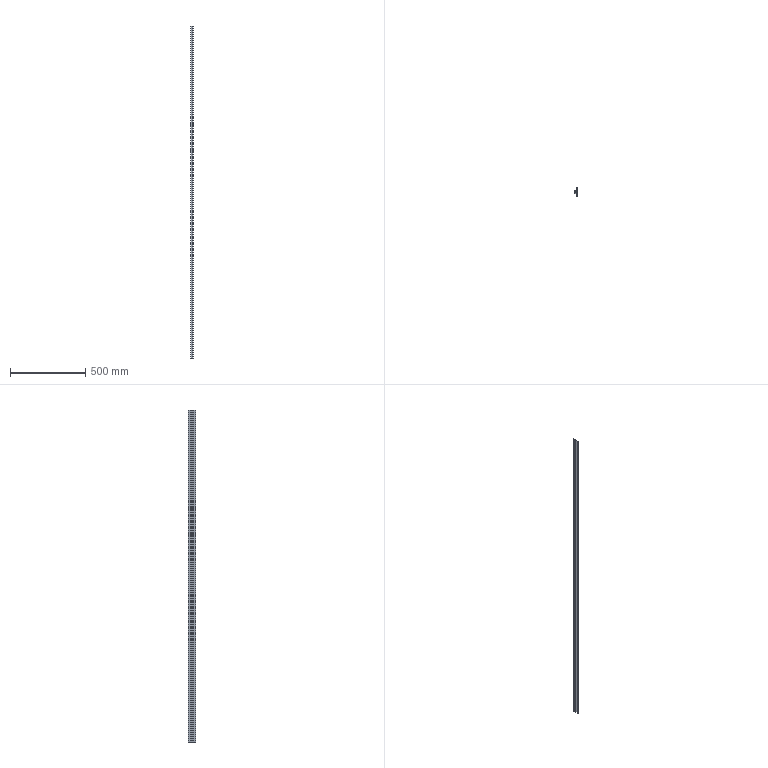Part | STEP file | Guide wheel mechanism revised.sldasm-Part-78 | 1 solid | 22 faces | box 14 x 50 x 2200 mm | volume 559680 mm3 | plane 22
STEP:
#1=CARTESIAN_POINT('',(0.,-7.,-1100.));
#2=VERTEX_POINT('',#1);
#3=CARTESIAN_POINT('',(-8.,-7.,-1100.));
#4=VERTEX_POINT('',#3);
#5=CARTESIAN_POINT('',(-8.,-7.,-1100.));
#6=DIRECTION('',(-1.,0.,0.));
#7=VECTOR('',#6,1000.);
#8=LINE('',#5,#7);
#9=EDGE_CURVE('',#2,#4,#8,.T.);
#10=ORIENTED_EDGE('',*,*,#9,.T.);
#11=CARTESIAN_POINT('',(-8.,-7.,1100.));
#12=VERTEX_POINT('',#11);
#13=CARTESIAN_POINT('',(-8.,-7.,1100.));
#14=DIRECTION('',(0.,0.,-1.));
#15=VECTOR('',#14,1000.);
#16=LINE('',#13,#15);
#17=EDGE_CURVE('',#12,#4,#16,.T.);
#18=ORIENTED_EDGE('',*,*,#17,.F.);
#19=CARTESIAN_POINT('',(0.,-7.,1100.));
#20=VERTEX_POINT('',#19);
#21=CARTESIAN_POINT('',(-8.,-7.,1100.));
#22=DIRECTION('',(-1.,0.,0.));
#23=VECTOR('',#22,1000.);
#24=LINE('',#21,#23);
#25=EDGE_CURVE('',#20,#12,#24,.T.);
#26=ORIENTED_EDGE('',*,*,#25,.F.);
#27=CARTESIAN_POINT('',(0.,-7.,1100.));
#28=DIRECTION('',(0.,0.,-1.));
#29=VECTOR('',#28,1000.);
#30=LINE('',#27,#29);
#31=EDGE_CURVE('',#20,#2,#30,.T.);
#32=ORIENTED_EDGE('',*,*,#31,.T.);
#33=EDGE_LOOP('',(#10,#18,#26,#32));
#34=FACE_OUTER_BOUND('',#33,.T.);
#35=CARTESIAN_POINT('',(-8.,-7.,1100.));
#36=DIRECTION('',(0.,-1.,0.));
#37=DIRECTION('',(1.,0.,0.));
#38=AXIS2_PLACEMENT_3D('',#35,#36,#37);
#39=PLANE('',#38);
#40=ADVANCED_FACE('',(#34),#39,.F.);
#41=CARTESIAN_POINT('',(-8.,-4.6,-1100.));
#42=VERTEX_POINT('',#41);
#43=CARTESIAN_POINT('',(-8.,-4.6,-1100.));
#44=DIRECTION('',(0.,1.,0.));
#45=VECTOR('',#44,1000.);
#46=LINE('',#43,#45);
#47=EDGE_CURVE('',#4,#42,#46,.T.);
#48=ORIENTED_EDGE('',*,*,#47,.T.);
#49=CARTESIAN_POINT('',(-8.,-4.6,1100.));
#50=VERTEX_POINT('',#49);
#51=CARTESIAN_POINT('',(-8.,-4.6,1100.));
#52=DIRECTION('',(0.,0.,-1.));
#53=VECTOR('',#52,1000.);
#54=LINE('',#51,#53);
#55=EDGE_CURVE('',#50,#42,#54,.T.);
#56=ORIENTED_EDGE('',*,*,#55,.F.);
#57=CARTESIAN_POINT('',(-8.,-4.6,1100.));
#58=DIRECTION('',(0.,1.,0.));
#59=VECTOR('',#58,1000.);
#60=LINE('',#57,#59);
#61=EDGE_CURVE('',#12,#50,#60,.T.);
#62=ORIENTED_EDGE('',*,*,#61,.F.);
#63=ORIENTED_EDGE('',*,*,#17,.T.);
#64=EDGE_LOOP('',(#48,#56,#62,#63));
#65=FACE_OUTER_BOUND('',#64,.T.);
#66=CARTESIAN_POINT('',(-8.,-4.6,1100.));
#67=DIRECTION('',(-1.,0.,0.));
#68=DIRECTION('',(0.,0.,1.));
#69=AXIS2_PLACEMENT_3D('',#66,#67,#68);
#70=PLANE('',#69);
#71=ADVANCED_FACE('',(#65),#70,.F.);
#72=CARTESIAN_POINT('',(-11.,-4.6,-1100.));
#73=VERTEX_POINT('',#72);
#74=CARTESIAN_POINT('',(-11.,-4.6,-1100.));
#75=DIRECTION('',(-1.,0.,0.));
#76=VECTOR('',#75,1000.);
#77=LINE('',#74,#76);
#78=EDGE_CURVE('',#42,#73,#77,.T.);
#79=ORIENTED_EDGE('',*,*,#78,.T.);
#80=CARTESIAN_POINT('',(-11.,-4.6,1100.));
#81=VERTEX_POINT('',#80);
#82=CARTESIAN_POINT('',(-11.,-4.6,1100.));
#83=DIRECTION('',(0.,0.,-1.));
#84=VECTOR('',#83,1000.);
#85=LINE('',#82,#84);
#86=EDGE_CURVE('',#81,#73,#85,.T.);
#87=ORIENTED_EDGE('',*,*,#86,.F.);
#88=CARTESIAN_POINT('',(-11.,-4.6,1100.));
#89=DIRECTION('',(-1.,0.,0.));
#90=VECTOR('',#89,1000.);
#91=LINE('',#88,#90);
#92=EDGE_CURVE('',#50,#81,#91,.T.);
#93=ORIENTED_EDGE('',*,*,#92,.F.);
#94=ORIENTED_EDGE('',*,*,#55,.T.);
#95=EDGE_LOOP('',(#79,#87,#93,#94));
#96=FACE_OUTER_BOUND('',#95,.T.);
#97=CARTESIAN_POINT('',(-11.,-4.6,1100.));
#98=DIRECTION('',(0.,-1.,0.));
#99=DIRECTION('',(0.,0.,-1.));
#100=AXIS2_PLACEMENT_3D('',#97,#98,#99);
#101=PLANE('',#100);
#102=ADVANCED_FACE('',(#96),#101,.F.);
#103=CARTESIAN_POINT('',(-11.,-10.,-1100.));
#104=VERTEX_POINT('',#103);
#105=CARTESIAN_POINT('',(-11.,-10.,-1100.));
#106=DIRECTION('',(0.,-1.,0.));
#107=VECTOR('',#106,1000.);
#108=LINE('',#105,#107);
#109=EDGE_CURVE('',#73,#104,#108,.T.);
#110=ORIENTED_EDGE('',*,*,#109,.T.);
#111=CARTESIAN_POINT('',(-11.,-10.,1100.));
#112=VERTEX_POINT('',#111);
#113=CARTESIAN_POINT('',(-11.,-10.,1100.));
#114=DIRECTION('',(0.,0.,-1.));
#115=VECTOR('',#114,1000.);
#116=LINE('',#113,#115);
#117=EDGE_CURVE('',#112,#104,#116,.T.);
#118=ORIENTED_EDGE('',*,*,#117,.F.);
#119=CARTESIAN_POINT('',(-11.,-10.,1100.));
#120=DIRECTION('',(0.,-1.,0.));
#121=VECTOR('',#120,1000.);
#122=LINE('',#119,#121);
#123=EDGE_CURVE('',#81,#112,#122,.T.);
#124=ORIENTED_EDGE('',*,*,#123,.F.);
#125=ORIENTED_EDGE('',*,*,#86,.T.);
#126=EDGE_LOOP('',(#110,#118,#124,#125));
#127=FACE_OUTER_BOUND('',#126,.T.);
#128=CARTESIAN_POINT('',(-11.,-10.,1100.));
#129=DIRECTION('',(1.,0.,0.));
#130=DIRECTION('',(0.,1.,0.));
#131=AXIS2_PLACEMENT_3D('',#128,#129,#130);
#132=PLANE('',#131);
#133=ADVANCED_FACE('',(#127),#132,.F.);
#134=CARTESIAN_POINT('',(0.,-10.,-1100.));
#135=VERTEX_POINT('',#134);
#136=CARTESIAN_POINT('',(0.,-10.,-1100.));
#137=DIRECTION('',(1.,0.,0.));
#138=VECTOR('',#137,1000.);
#139=LINE('',#136,#138);
#140=EDGE_CURVE('',#104,#135,#139,.T.);
#141=ORIENTED_EDGE('',*,*,#140,.T.);
#142=CARTESIAN_POINT('',(0.,-10.,1100.));
#143=VERTEX_POINT('',#142);
#144=CARTESIAN_POINT('',(0.,-10.,1100.));
#145=DIRECTION('',(0.,0.,-1.));
#146=VECTOR('',#145,1000.);
#147=LINE('',#144,#146);
#148=EDGE_CURVE('',#143,#135,#147,.T.);
#149=ORIENTED_EDGE('',*,*,#148,.F.);
#150=CARTESIAN_POINT('',(0.,-10.,1100.));
#151=DIRECTION('',(1.,0.,0.));
#152=VECTOR('',#151,1000.);
#153=LINE('',#150,#152);
#154=EDGE_CURVE('',#112,#143,#153,.T.);
#155=ORIENTED_EDGE('',*,*,#154,.F.);
#156=ORIENTED_EDGE('',*,*,#117,.T.);
#157=EDGE_LOOP('',(#141,#149,#155,#156));
#158=FACE_OUTER_BOUND('',#157,.T.);
#159=CARTESIAN_POINT('',(0.,-10.,1100.));
#160=DIRECTION('',(0.,1.,0.));
#161=DIRECTION('',(-1.,0.,0.));
#162=AXIS2_PLACEMENT_3D('',#159,#160,#161);
#163=PLANE('',#162);
#164=ADVANCED_FACE('',(#158),#163,.F.);
#165=CARTESIAN_POINT('',(0.,-21.,-1100.));
#166=VERTEX_POINT('',#165);
#167=CARTESIAN_POINT('',(0.,-21.,-1100.));
#168=DIRECTION('',(0.,-1.,0.));
#169=VECTOR('',#168,1000.);
#170=LINE('',#167,#169);
#171=EDGE_CURVE('',#135,#166,#170,.T.);
#172=ORIENTED_EDGE('',*,*,#171,.T.);
#173=CARTESIAN_POINT('',(0.,-21.,1100.));
#174=VERTEX_POINT('',#173);
#175=CARTESIAN_POINT('',(0.,-21.,1100.));
#176=DIRECTION('',(0.,0.,-1.));
#177=VECTOR('',#176,1000.);
#178=LINE('',#175,#177);
#179=EDGE_CURVE('',#174,#166,#178,.T.);
#180=ORIENTED_EDGE('',*,*,#179,.F.);
#181=CARTESIAN_POINT('',(0.,-21.,1100.));
#182=DIRECTION('',(0.,-1.,0.));
#183=VECTOR('',#182,1000.);
#184=LINE('',#181,#183);
#185=EDGE_CURVE('',#143,#174,#184,.T.);
#186=ORIENTED_EDGE('',*,*,#185,.F.);
#187=ORIENTED_EDGE('',*,*,#148,.T.);
#188=EDGE_LOOP('',(#172,#180,#186,#187));
#189=FACE_OUTER_BOUND('',#188,.T.);
#190=CARTESIAN_POINT('',(0.,-21.,1100.));
#191=DIRECTION('',(1.,0.,0.));
#192=DIRECTION('',(0.,1.,0.));
#193=AXIS2_PLACEMENT_3D('',#190,#191,#192);
#194=PLANE('',#193);
#195=ADVANCED_FACE('',(#189),#194,.F.);
#196=CARTESIAN_POINT('',(-3.,-21.,-1100.));
#197=VERTEX_POINT('',#196);
#198=CARTESIAN_POINT('',(-3.,-21.,-1100.));
#199=DIRECTION('',(-1.,0.,0.));
#200=VECTOR('',#199,1000.);
#201=LINE('',#198,#200);
#202=EDGE_CURVE('',#166,#197,#201,.T.);
#203=ORIENTED_EDGE('',*,*,#202,.T.);
#204=CARTESIAN_POINT('',(-3.,-21.,1100.));
#205=VERTEX_POINT('',#204);
#206=CARTESIAN_POINT('',(-3.,-21.,1100.));
#207=DIRECTION('',(0.,0.,-1.));
#208=VECTOR('',#207,1000.);
#209=LINE('',#206,#208);
#210=EDGE_CURVE('',#205,#197,#209,.T.);
#211=ORIENTED_EDGE('',*,*,#210,.F.);
#212=CARTESIAN_POINT('',(-3.,-21.,1100.));
#213=DIRECTION('',(-1.,0.,0.));
#214=VECTOR('',#213,1000.);
#215=LINE('',#212,#214);
#216=EDGE_CURVE('',#174,#205,#215,.T.);
#217=ORIENTED_EDGE('',*,*,#216,.F.);
#218=ORIENTED_EDGE('',*,*,#179,.T.);
#219=EDGE_LOOP('',(#203,#211,#217,#218));
#220=FACE_OUTER_BOUND('',#219,.T.);
#221=CARTESIAN_POINT('',(-3.,-21.,1100.));
#222=DIRECTION('',(0.,-1.,0.));
#223=DIRECTION('',(1.,0.,0.));
#224=AXIS2_PLACEMENT_3D('',#221,#222,#223);
#225=PLANE('',#224);
#226=ADVANCED_FACE('',(#220),#225,.F.);
#227=CARTESIAN_POINT('',(-3.,-25.,-1100.));
#228=VERTEX_POINT('',#227);
#229=CARTESIAN_POINT('',(-3.,-25.,-1100.));
#230=DIRECTION('',(0.,-1.,0.));
#231=VECTOR('',#230,1000.);
#232=LINE('',#229,#231);
#233=EDGE_CURVE('',#197,#228,#232,.T.);
#234=ORIENTED_EDGE('',*,*,#233,.T.);
#235=CARTESIAN_POINT('',(-3.,-25.,1100.));
#236=VERTEX_POINT('',#235);
#237=CARTESIAN_POINT('',(-3.,-25.,1100.));
#238=DIRECTION('',(0.,0.,-1.));
#239=VECTOR('',#238,1000.);
#240=LINE('',#237,#239);
#241=EDGE_CURVE('',#236,#228,#240,.T.);
#242=ORIENTED_EDGE('',*,*,#241,.F.);
#243=CARTESIAN_POINT('',(-3.,-25.,1100.));
#244=DIRECTION('',(0.,-1.,0.));
#245=VECTOR('',#244,1000.);
#246=LINE('',#243,#245);
#247=EDGE_CURVE('',#205,#236,#246,.T.);
#248=ORIENTED_EDGE('',*,*,#247,.F.);
#249=ORIENTED_EDGE('',*,*,#210,.T.);
#250=EDGE_LOOP('',(#234,#242,#248,#249));
#251=FACE_OUTER_BOUND('',#250,.T.);
#252=CARTESIAN_POINT('',(-3.,-25.,1100.));
#253=DIRECTION('',(1.,0.,0.));
#254=DIRECTION('',(0.,0.,-1.));
#255=AXIS2_PLACEMENT_3D('',#252,#253,#254);
#256=PLANE('',#255);
#257=ADVANCED_FACE('',(#251),#256,.F.);
#258=CARTESIAN_POINT('',(3.,-25.,-1100.));
#259=VERTEX_POINT('',#258);
#260=CARTESIAN_POINT('',(3.,-25.,-1100.));
#261=DIRECTION('',(1.,0.,0.));
#262=VECTOR('',#261,1000.);
#263=LINE('',#260,#262);
#264=EDGE_CURVE('',#228,#259,#263,.T.);
#265=ORIENTED_EDGE('',*,*,#264,.T.);
#266=CARTESIAN_POINT('',(3.,-25.,1100.));
#267=VERTEX_POINT('',#266);
#268=CARTESIAN_POINT('',(3.,-25.,1100.));
#269=DIRECTION('',(0.,0.,-1.));
#270=VECTOR('',#269,1000.);
#271=LINE('',#268,#270);
#272=EDGE_CURVE('',#267,#259,#271,.T.);
#273=ORIENTED_EDGE('',*,*,#272,.F.);
#274=CARTESIAN_POINT('',(3.,-25.,1100.));
#275=DIRECTION('',(1.,0.,0.));
#276=VECTOR('',#275,1000.);
#277=LINE('',#274,#276);
#278=EDGE_CURVE('',#236,#267,#277,.T.);
#279=ORIENTED_EDGE('',*,*,#278,.F.);
#280=ORIENTED_EDGE('',*,*,#241,.T.);
#281=EDGE_LOOP('',(#265,#273,#279,#280));
#282=FACE_OUTER_BOUND('',#281,.T.);
#283=CARTESIAN_POINT('',(3.,-25.,1100.));
#284=DIRECTION('',(0.,1.,0.));
#285=DIRECTION('',(0.,0.,1.));
#286=AXIS2_PLACEMENT_3D('',#283,#284,#285);
#287=PLANE('',#286);
#288=ADVANCED_FACE('',(#282),#287,.F.);
#289=CARTESIAN_POINT('',(3.,25.,-1100.));
#290=VERTEX_POINT('',#289);
#291=CARTESIAN_POINT('',(3.,-25.,-1100.));
#292=DIRECTION('',(0.,1.,0.));
#293=VECTOR('',#292,1000.);
#294=LINE('',#291,#293);
#295=EDGE_CURVE('',#259,#290,#294,.T.);
#296=ORIENTED_EDGE('',*,*,#295,.T.);
#297=CARTESIAN_POINT('',(3.,25.,1100.));
#298=VERTEX_POINT('',#297);
#299=CARTESIAN_POINT('',(3.,25.,1100.));
#300=DIRECTION('',(0.,0.,-1.));
#301=VECTOR('',#300,1000.);
#302=LINE('',#299,#301);
#303=EDGE_CURVE('',#298,#290,#302,.T.);
#304=ORIENTED_EDGE('',*,*,#303,.F.);
#305=CARTESIAN_POINT('',(3.,-25.,1100.));
#306=DIRECTION('',(0.,1.,0.));
#307=VECTOR('',#306,1000.);
#308=LINE('',#305,#307);
#309=EDGE_CURVE('',#267,#298,#308,.T.);
#310=ORIENTED_EDGE('',*,*,#309,.F.);
#311=ORIENTED_EDGE('',*,*,#272,.T.);
#312=EDGE_LOOP('',(#296,#304,#310,#311));
#313=FACE_OUTER_BOUND('',#312,.T.);
#314=CARTESIAN_POINT('',(3.,-25.,1100.));
#315=DIRECTION('',(-1.,0.,0.));
#316=DIRECTION('',(0.,0.,1.));
#317=AXIS2_PLACEMENT_3D('',#314,#315,#316);
#318=PLANE('',#317);
#319=ADVANCED_FACE('',(#313),#318,.F.);
#320=CARTESIAN_POINT('',(-3.,25.,-1100.));
#321=VERTEX_POINT('',#320);
#322=CARTESIAN_POINT('',(3.,25.,-1100.));
#323=DIRECTION('',(-1.,0.,0.));
#324=VECTOR('',#323,1000.);
#325=LINE('',#322,#324);
#326=EDGE_CURVE('',#290,#321,#325,.T.);
#327=ORIENTED_EDGE('',*,*,#326,.T.);
#328=CARTESIAN_POINT('',(-3.,25.,1100.));
#329=VERTEX_POINT('',#328);
#330=CARTESIAN_POINT('',(-3.,25.,1100.));
#331=DIRECTION('',(0.,0.,-1.));
#332=VECTOR('',#331,1000.);
#333=LINE('',#330,#332);
#334=EDGE_CURVE('',#329,#321,#333,.T.);
#335=ORIENTED_EDGE('',*,*,#334,.F.);
#336=CARTESIAN_POINT('',(3.,25.,1100.));
#337=DIRECTION('',(-1.,0.,0.));
#338=VECTOR('',#337,1000.);
#339=LINE('',#336,#338);
#340=EDGE_CURVE('',#298,#329,#339,.T.);
#341=ORIENTED_EDGE('',*,*,#340,.F.);
#342=ORIENTED_EDGE('',*,*,#303,.T.);
#343=EDGE_LOOP('',(#327,#335,#341,#342));
#344=FACE_OUTER_BOUND('',#343,.T.);
#345=CARTESIAN_POINT('',(3.,25.,1100.));
#346=DIRECTION('',(0.,-1.,0.));
#347=DIRECTION('',(0.,0.,-1.));
#348=AXIS2_PLACEMENT_3D('',#345,#346,#347);
#349=PLANE('',#348);
#350=ADVANCED_FACE('',(#344),#349,.F.);
#351=CARTESIAN_POINT('',(-3.,21.,-1100.));
#352=VERTEX_POINT('',#351);
#353=CARTESIAN_POINT('',(-3.,25.,-1100.));
#354=DIRECTION('',(0.,-1.,0.));
#355=VECTOR('',#354,1000.);
#356=LINE('',#353,#355);
#357=EDGE_CURVE('',#321,#352,#356,.T.);
#358=ORIENTED_EDGE('',*,*,#357,.T.);
#359=CARTESIAN_POINT('',(-3.,21.,1100.));
#360=VERTEX_POINT('',#359);
#361=CARTESIAN_POINT('',(-3.,21.,1100.));
#362=DIRECTION('',(0.,0.,-1.));
#363=VECTOR('',#362,1000.);
#364=LINE('',#361,#363);
#365=EDGE_CURVE('',#360,#352,#364,.T.);
#366=ORIENTED_EDGE('',*,*,#365,.F.);
#367=CARTESIAN_POINT('',(-3.,25.,1100.));
#368=DIRECTION('',(0.,-1.,0.));
#369=VECTOR('',#368,1000.);
#370=LINE('',#367,#369);
#371=EDGE_CURVE('',#329,#360,#370,.T.);
#372=ORIENTED_EDGE('',*,*,#371,.F.);
#373=ORIENTED_EDGE('',*,*,#334,.T.);
#374=EDGE_LOOP('',(#358,#366,#372,#373));
#375=FACE_OUTER_BOUND('',#374,.T.);
#376=CARTESIAN_POINT('',(-3.,25.,1100.));
#377=DIRECTION('',(1.,0.,0.));
#378=DIRECTION('',(0.,0.,-1.));
#379=AXIS2_PLACEMENT_3D('',#376,#377,#378);
#380=PLANE('',#379);
#381=ADVANCED_FACE('',(#375),#380,.F.);
#382=CARTESIAN_POINT('',(0.,21.,-1100.));
#383=VERTEX_POINT('',#382);
#384=CARTESIAN_POINT('',(-3.,21.,-1100.));
#385=DIRECTION('',(1.,0.,0.));
#386=VECTOR('',#385,1000.);
#387=LINE('',#384,#386);
#388=EDGE_CURVE('',#352,#383,#387,.T.);
#389=ORIENTED_EDGE('',*,*,#388,.T.);
#390=CARTESIAN_POINT('',(0.,21.,1100.));
#391=VERTEX_POINT('',#390);
#392=CARTESIAN_POINT('',(0.,21.,1100.));
#393=DIRECTION('',(0.,0.,-1.));
#394=VECTOR('',#393,1000.);
#395=LINE('',#392,#394);
#396=EDGE_CURVE('',#391,#383,#395,.T.);
#397=ORIENTED_EDGE('',*,*,#396,.F.);
#398=CARTESIAN_POINT('',(-3.,21.,1100.));
#399=DIRECTION('',(1.,0.,0.));
#400=VECTOR('',#399,1000.);
#401=LINE('',#398,#400);
#402=EDGE_CURVE('',#360,#391,#401,.T.);
#403=ORIENTED_EDGE('',*,*,#402,.F.);
#404=ORIENTED_EDGE('',*,*,#365,.T.);
#405=EDGE_LOOP('',(#389,#397,#403,#404));
#406=FACE_OUTER_BOUND('',#405,.T.);
#407=CARTESIAN_POINT('',(-3.,21.,1100.));
#408=DIRECTION('',(0.,1.,0.));
#409=DIRECTION('',(-1.,0.,0.));
#410=AXIS2_PLACEMENT_3D('',#407,#408,#409);
#411=PLANE('',#410);
#412=ADVANCED_FACE('',(#406),#411,.F.);
#413=CARTESIAN_POINT('',(0.,10.,-1100.));
#414=VERTEX_POINT('',#413);
#415=CARTESIAN_POINT('',(0.,21.,-1100.));
#416=DIRECTION('',(0.,-1.,0.));
#417=VECTOR('',#416,1000.);
#418=LINE('',#415,#417);
#419=EDGE_CURVE('',#383,#414,#418,.T.);
#420=ORIENTED_EDGE('',*,*,#419,.T.);
#421=CARTESIAN_POINT('',(0.,10.,1100.));
#422=VERTEX_POINT('',#421);
#423=CARTESIAN_POINT('',(0.,10.,1100.));
#424=DIRECTION('',(0.,0.,-1.));
#425=VECTOR('',#424,1000.);
#426=LINE('',#423,#425);
#427=EDGE_CURVE('',#422,#414,#426,.T.);
#428=ORIENTED_EDGE('',*,*,#427,.F.);
#429=CARTESIAN_POINT('',(0.,21.,1100.));
#430=DIRECTION('',(0.,-1.,0.));
#431=VECTOR('',#430,1000.);
#432=LINE('',#429,#431);
#433=EDGE_CURVE('',#391,#422,#432,.T.);
#434=ORIENTED_EDGE('',*,*,#433,.F.);
#435=ORIENTED_EDGE('',*,*,#396,.T.);
#436=EDGE_LOOP('',(#420,#428,#434,#435));
#437=FACE_OUTER_BOUND('',#436,.T.);
#438=CARTESIAN_POINT('',(0.,21.,1100.));
#439=DIRECTION('',(1.,0.,0.));
#440=DIRECTION('',(0.,1.,0.));
#441=AXIS2_PLACEMENT_3D('',#438,#439,#440);
#442=PLANE('',#441);
#443=ADVANCED_FACE('',(#437),#442,.F.);
#444=CARTESIAN_POINT('',(-11.,10.,-1100.));
#445=VERTEX_POINT('',#444);
#446=CARTESIAN_POINT('',(0.,10.,-1100.));
#447=DIRECTION('',(-1.,0.,0.));
#448=VECTOR('',#447,1000.);
#449=LINE('',#446,#448);
#450=EDGE_CURVE('',#414,#445,#449,.T.);
#451=ORIENTED_EDGE('',*,*,#450,.T.);
#452=CARTESIAN_POINT('',(-11.,10.,1100.));
#453=VERTEX_POINT('',#452);
#454=CARTESIAN_POINT('',(-11.,10.,1100.));
#455=DIRECTION('',(0.,0.,-1.));
#456=VECTOR('',#455,1000.);
#457=LINE('',#454,#456);
#458=EDGE_CURVE('',#453,#445,#457,.T.);
#459=ORIENTED_EDGE('',*,*,#458,.F.);
#460=CARTESIAN_POINT('',(0.,10.,1100.));
#461=DIRECTION('',(-1.,0.,0.));
#462=VECTOR('',#461,1000.);
#463=LINE('',#460,#462);
#464=EDGE_CURVE('',#422,#453,#463,.T.);
#465=ORIENTED_EDGE('',*,*,#464,.F.);
#466=ORIENTED_EDGE('',*,*,#427,.T.);
#467=EDGE_LOOP('',(#451,#459,#465,#466));
#468=FACE_OUTER_BOUND('',#467,.T.);
#469=CARTESIAN_POINT('',(0.,10.,1100.));
#470=DIRECTION('',(0.,-1.,0.));
#471=DIRECTION('',(1.,0.,0.));
#472=AXIS2_PLACEMENT_3D('',#469,#470,#471);
#473=PLANE('',#472);
#474=ADVANCED_FACE('',(#468),#473,.F.);
#475=CARTESIAN_POINT('',(-11.,4.6,-1100.));
#476=VERTEX_POINT('',#475);
#477=CARTESIAN_POINT('',(-11.,10.,-1100.));
#478=DIRECTION('',(0.,-1.,0.));
#479=VECTOR('',#478,1000.);
#480=LINE('',#477,#479);
#481=EDGE_CURVE('',#445,#476,#480,.T.);
#482=ORIENTED_EDGE('',*,*,#481,.T.);
#483=CARTESIAN_POINT('',(-11.,4.6,1100.));
#484=VERTEX_POINT('',#483);
#485=CARTESIAN_POINT('',(-11.,4.6,1100.));
#486=DIRECTION('',(0.,0.,-1.));
#487=VECTOR('',#486,1000.);
#488=LINE('',#485,#487);
#489=EDGE_CURVE('',#484,#476,#488,.T.);
#490=ORIENTED_EDGE('',*,*,#489,.F.);
#491=CARTESIAN_POINT('',(-11.,10.,1100.));
#492=DIRECTION('',(0.,-1.,0.));
#493=VECTOR('',#492,1000.);
#494=LINE('',#491,#493);
#495=EDGE_CURVE('',#453,#484,#494,.T.);
#496=ORIENTED_EDGE('',*,*,#495,.F.);
#497=ORIENTED_EDGE('',*,*,#458,.T.);
#498=EDGE_LOOP('',(#482,#490,#496,#497));
#499=FACE_OUTER_BOUND('',#498,.T.);
#500=CARTESIAN_POINT('',(-11.,10.,1100.));
#501=DIRECTION('',(1.,0.,0.));
#502=DIRECTION('',(0.,1.,0.));
#503=AXIS2_PLACEMENT_3D('',#500,#501,#502);
#504=PLANE('',#503);
#505=ADVANCED_FACE('',(#499),#504,.F.);
#506=CARTESIAN_POINT('',(-8.,4.6,-1100.));
#507=VERTEX_POINT('',#506);
#508=CARTESIAN_POINT('',(-11.,4.6,-1100.));
#509=DIRECTION('',(1.,0.,0.));
#510=VECTOR('',#509,1000.);
#511=LINE('',#508,#510);
#512=EDGE_CURVE('',#476,#507,#511,.T.);
#513=ORIENTED_EDGE('',*,*,#512,.T.);
#514=CARTESIAN_POINT('',(-8.,4.6,1100.));
#515=VERTEX_POINT('',#514);
#516=CARTESIAN_POINT('',(-8.,4.6,1100.));
#517=DIRECTION('',(0.,0.,-1.));
#518=VECTOR('',#517,1000.);
#519=LINE('',#516,#518);
#520=EDGE_CURVE('',#515,#507,#519,.T.);
#521=ORIENTED_EDGE('',*,*,#520,.F.);
#522=CARTESIAN_POINT('',(-11.,4.6,1100.));
#523=DIRECTION('',(1.,0.,0.));
#524=VECTOR('',#523,1000.);
#525=LINE('',#522,#524);
#526=EDGE_CURVE('',#484,#515,#525,.T.);
#527=ORIENTED_EDGE('',*,*,#526,.F.);
#528=ORIENTED_EDGE('',*,*,#489,.T.);
#529=EDGE_LOOP('',(#513,#521,#527,#528));
#530=FACE_OUTER_BOUND('',#529,.T.);
#531=CARTESIAN_POINT('',(-11.,4.6,1100.));
#532=DIRECTION('',(0.,1.,0.));
#533=DIRECTION('',(0.,0.,1.));
#534=AXIS2_PLACEMENT_3D('',#531,#532,#533);
#535=PLANE('',#534);
#536=ADVANCED_FACE('',(#530),#535,.F.);
#537=CARTESIAN_POINT('',(-8.,7.,-1100.));
#538=VERTEX_POINT('',#537);
#539=CARTESIAN_POINT('',(-8.,4.6,-1100.));
#540=DIRECTION('',(0.,1.,0.));
#541=VECTOR('',#540,1000.);
#542=LINE('',#539,#541);
#543=EDGE_CURVE('',#507,#538,#542,.T.);
#544=ORIENTED_EDGE('',*,*,#543,.T.);
#545=CARTESIAN_POINT('',(-8.,7.,1100.));
#546=VERTEX_POINT('',#545);
#547=CARTESIAN_POINT('',(-8.,7.,1100.));
#548=DIRECTION('',(0.,0.,-1.));
#549=VECTOR('',#548,1000.);
#550=LINE('',#547,#549);
#551=EDGE_CURVE('',#546,#538,#550,.T.);
#552=ORIENTED_EDGE('',*,*,#551,.F.);
#553=CARTESIAN_POINT('',(-8.,4.6,1100.));
#554=DIRECTION('',(0.,1.,0.));
#555=VECTOR('',#554,1000.);
#556=LINE('',#553,#555);
#557=EDGE_CURVE('',#515,#546,#556,.T.);
#558=ORIENTED_EDGE('',*,*,#557,.F.);
#559=ORIENTED_EDGE('',*,*,#520,.T.);
#560=EDGE_LOOP('',(#544,#552,#558,#559));
#561=FACE_OUTER_BOUND('',#560,.T.);
#562=CARTESIAN_POINT('',(-8.,4.6,1100.));
#563=DIRECTION('',(-1.,0.,0.));
#564=DIRECTION('',(0.,0.,1.));
#565=AXIS2_PLACEMENT_3D('',#562,#563,#564);
#566=PLANE('',#565);
#567=ADVANCED_FACE('',(#561),#566,.F.);
#568=CARTESIAN_POINT('',(0.,7.,-1100.));
#569=VERTEX_POINT('',#568);
#570=CARTESIAN_POINT('',(-8.,7.,-1100.));
#571=DIRECTION('',(1.,0.,0.));
#572=VECTOR('',#571,1000.);
#573=LINE('',#570,#572);
#574=EDGE_CURVE('',#538,#569,#573,.T.);
#575=ORIENTED_EDGE('',*,*,#574,.T.);
#576=CARTESIAN_POINT('',(0.,7.,1100.));
#577=VERTEX_POINT('',#576);
#578=CARTESIAN_POINT('',(0.,7.,1100.));
#579=DIRECTION('',(0.,0.,-1.));
#580=VECTOR('',#579,1000.);
#581=LINE('',#578,#580);
#582=EDGE_CURVE('',#577,#569,#581,.T.);
#583=ORIENTED_EDGE('',*,*,#582,.F.);
#584=CARTESIAN_POINT('',(-8.,7.,1100.));
#585=DIRECTION('',(1.,0.,0.));
#586=VECTOR('',#585,1000.);
#587=LINE('',#584,#586);
#588=EDGE_CURVE('',#546,#577,#587,.T.);
#589=ORIENTED_EDGE('',*,*,#588,.F.);
#590=ORIENTED_EDGE('',*,*,#551,.T.);
#591=EDGE_LOOP('',(#575,#583,#589,#590));
#592=FACE_OUTER_BOUND('',#591,.T.);
#593=CARTESIAN_POINT('',(-8.,7.,1100.));
#594=DIRECTION('',(0.,1.,0.));
#595=DIRECTION('',(-1.,0.,0.));
#596=AXIS2_PLACEMENT_3D('',#593,#594,#595);
#597=PLANE('',#596);
#598=ADVANCED_FACE('',(#592),#597,.F.);
#599=CARTESIAN_POINT('',(0.,7.,-1100.));
#600=DIRECTION('',(0.,-1.,0.));
#601=VECTOR('',#600,1000.);
#602=LINE('',#599,#601);
#603=EDGE_CURVE('',#569,#2,#602,.T.);
#604=ORIENTED_EDGE('',*,*,#603,.T.);
#605=ORIENTED_EDGE('',*,*,#31,.F.);
#606=CARTESIAN_POINT('',(0.,7.,1100.));
#607=DIRECTION('',(0.,-1.,0.));
#608=VECTOR('',#607,1000.);
#609=LINE('',#606,#608);
#610=EDGE_CURVE('',#577,#20,#609,.T.);
#611=ORIENTED_EDGE('',*,*,#610,.F.);
#612=ORIENTED_EDGE('',*,*,#582,.T.);
#613=EDGE_LOOP('',(#604,#605,#611,#612));
#614=FACE_OUTER_BOUND('',#613,.T.);
#615=CARTESIAN_POINT('',(0.,7.,1100.));
#616=DIRECTION('',(1.,0.,0.));
#617=DIRECTION('',(0.,0.,-1.));
#618=AXIS2_PLACEMENT_3D('',#615,#616,#617);
#619=PLANE('',#618);
#620=ADVANCED_FACE('',(#614),#619,.F.);
#621=ORIENTED_EDGE('',*,*,#25,.T.);
#622=ORIENTED_EDGE('',*,*,#61,.T.);
#623=ORIENTED_EDGE('',*,*,#92,.T.);
#624=ORIENTED_EDGE('',*,*,#123,.T.);
#625=ORIENTED_EDGE('',*,*,#154,.T.);
#626=ORIENTED_EDGE('',*,*,#185,.T.);
#627=ORIENTED_EDGE('',*,*,#216,.T.);
#628=ORIENTED_EDGE('',*,*,#247,.T.);
#629=ORIENTED_EDGE('',*,*,#278,.T.);
#630=ORIENTED_EDGE('',*,*,#309,.T.);
#631=ORIENTED_EDGE('',*,*,#340,.T.);
#632=ORIENTED_EDGE('',*,*,#371,.T.);
#633=ORIENTED_EDGE('',*,*,#402,.T.);
#634=ORIENTED_EDGE('',*,*,#433,.T.);
#635=ORIENTED_EDGE('',*,*,#464,.T.);
#636=ORIENTED_EDGE('',*,*,#495,.T.);
#637=ORIENTED_EDGE('',*,*,#526,.T.);
#638=ORIENTED_EDGE('',*,*,#557,.T.);
#639=ORIENTED_EDGE('',*,*,#588,.T.);
#640=ORIENTED_EDGE('',*,*,#610,.T.);
#641=EDGE_LOOP('',(#621,#622,#623,#624,#625,#626,#627,#628,#629,#630,#631,#632,#633,#634,#635,#636,#637,#638,#639,#640));
#642=FACE_OUTER_BOUND('',#641,.T.);
#643=CARTESIAN_POINT('',(0.,0.,1100.));
#644=DIRECTION('',(0.,0.,-1.));
#645=DIRECTION('',(-1.,0.,0.));
#646=AXIS2_PLACEMENT_3D('',#643,#644,#645);
#647=PLANE('',#646);
#648=ADVANCED_FACE('',(#642),#647,.F.);
#649=ORIENTED_EDGE('',*,*,#9,.F.);
#650=ORIENTED_EDGE('',*,*,#603,.F.);
#651=ORIENTED_EDGE('',*,*,#574,.F.);
#652=ORIENTED_EDGE('',*,*,#543,.F.);
#653=ORIENTED_EDGE('',*,*,#512,.F.);
#654=ORIENTED_EDGE('',*,*,#481,.F.);
#655=ORIENTED_EDGE('',*,*,#450,.F.);
#656=ORIENTED_EDGE('',*,*,#419,.F.);
#657=ORIENTED_EDGE('',*,*,#388,.F.);
#658=ORIENTED_EDGE('',*,*,#357,.F.);
#659=ORIENTED_EDGE('',*,*,#326,.F.);
#660=ORIENTED_EDGE('',*,*,#295,.F.);
#661=ORIENTED_EDGE('',*,*,#264,.F.);
#662=ORIENTED_EDGE('',*,*,#233,.F.);
#663=ORIENTED_EDGE('',*,*,#202,.F.);
#664=ORIENTED_EDGE('',*,*,#171,.F.);
#665=ORIENTED_EDGE('',*,*,#140,.F.);
#666=ORIENTED_EDGE('',*,*,#109,.F.);
#667=ORIENTED_EDGE('',*,*,#78,.F.);
#668=ORIENTED_EDGE('',*,*,#47,.F.);
#669=EDGE_LOOP('',(#649,#650,#651,#652,#653,#654,#655,#656,#657,#658,#659,#660,#661,#662,#663,#664,#665,#666,#667,#668));
#670=FACE_OUTER_BOUND('',#669,.T.);
#671=CARTESIAN_POINT('',(0.,0.,-1100.));
#672=DIRECTION('',(0.,0.,-1.));
#673=DIRECTION('',(-1.,0.,0.));
#674=AXIS2_PLACEMENT_3D('',#671,#672,#673);
#675=PLANE('',#674);
#676=ADVANCED_FACE('',(#670),#675,.T.);
#677=CLOSED_SHELL('',(#40,#71,#102,#133,#164,#195,#226,#257,#288,#319,#350,#381,#412,#443,#474,#505,#536,#567,#598,#620,#648,#676));
#678=MANIFOLD_SOLID_BREP('',#677);
#679=CARTESIAN_POINT('',(0.,0.,0.));
#680=DIRECTION('',(0.,0.,1.));
#681=DIRECTION('',(1.,0.,0.));
#682=AXIS2_PLACEMENT_3D('',#679,#680,#681);
#683=(LENGTH_UNIT()NAMED_UNIT(*)SI_UNIT(.MILLI.,.METRE.));
#684=UNCERTAINTY_MEASURE_WITH_UNIT(LENGTH_MEASURE(0.00001),#683,'','');
#685=(NAMED_UNIT(*)PLANE_ANGLE_UNIT()SI_UNIT($,.RADIAN.));
#686=(NAMED_UNIT(*)SI_UNIT($,.STERADIAN.)SOLID_ANGLE_UNIT());
#687=(GEOMETRIC_REPRESENTATION_CONTEXT(3)GLOBAL_UNCERTAINTY_ASSIGNED_CONTEXT((#684))GLOBAL_UNIT_ASSIGNED_CONTEXT((#683,#685,#686))REPRESENTATION_CONTEXT('',''));
#688=ADVANCED_BREP_SHAPE_REPRESENTATION('',(#678,#682),#687);